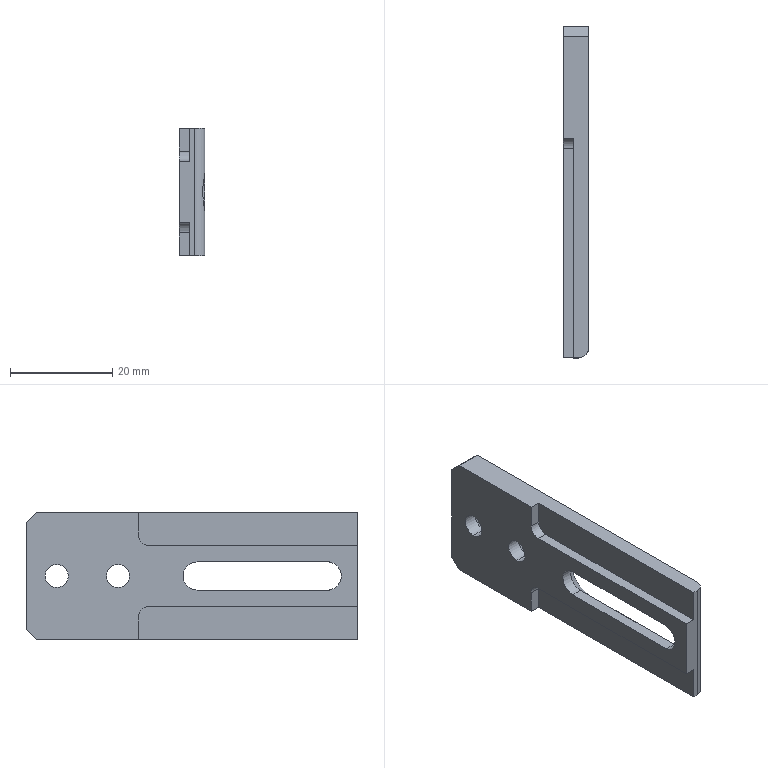Part | STEP file | 0-09-19 Support plate connecting plate | 1 solid | 35 faces | box 5 x 65 x 25 mm | volume 5596 mm3 | plane 20 | cylinder 9 | cone 6 | commonest cylinder face diameters 4.5 x4 4 x3 5.5 x2